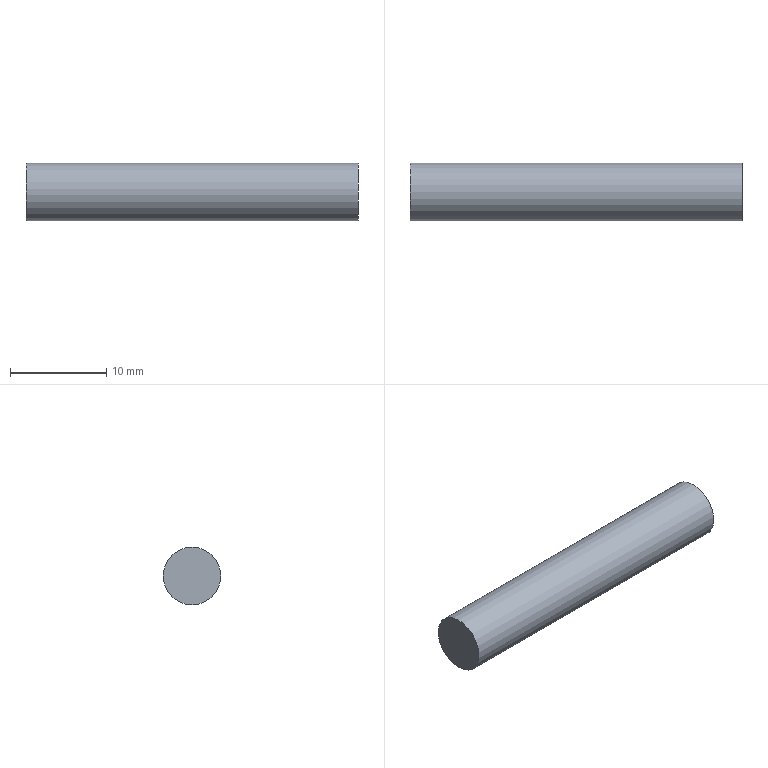Part | NX | features solid 2 | 1 solid | 3 faces | box 34.5 x 6 x 6 mm | volume 975.465 mm3 | plane 2 | cylinder 1 | commonest cylinder face diameters 6 x1
STEP:
#1=CARTESIAN_POINT('',(-125.,-72.,-32.));
#2=VERTEX_POINT('',#1);
#3=CARTESIAN_POINT('',(-125.,-72.,-35.));
#4=DIRECTION('',(-1.,0.,0.));
#5=DIRECTION('',(0.,0.,1.));
#6=AXIS2_PLACEMENT_3D('',#3,#4,#5);
#7=CIRCLE('',#6,3.);
#8=EDGE_CURVE('',#2,#2,#7,.F.);
#9=ORIENTED_EDGE('',*,*,#8,.T.);
#10=EDGE_LOOP('',(#9));
#11=FACE_BOUND('',#10,.T.);
#12=CARTESIAN_POINT('',(-90.5,-72.,-32.));
#13=VERTEX_POINT('',#12);
#14=CARTESIAN_POINT('',(-90.5,-72.,-35.));
#15=DIRECTION('',(-1.,0.,0.));
#16=DIRECTION('',(0.,0.,1.));
#17=AXIS2_PLACEMENT_3D('',#14,#15,#16);
#18=CIRCLE('',#17,3.);
#19=EDGE_CURVE('',#13,#13,#18,.F.);
#20=ORIENTED_EDGE('',*,*,#19,.F.);
#21=EDGE_LOOP('',(#20));
#22=FACE_BOUND('',#21,.T.);
#23=CARTESIAN_POINT('',(-125.,-72.,-35.));
#24=DIRECTION('',(1.,0.,0.));
#25=DIRECTION('',(0.,0.,1.));
#26=AXIS2_PLACEMENT_3D('',#23,#24,#25);
#27=CYLINDRICAL_SURFACE('',#26,3.);
#28=ADVANCED_FACE('',(#11,#22),#27,.T.);
#29=ORIENTED_EDGE('',*,*,#8,.F.);
#30=EDGE_LOOP('',(#29));
#31=FACE_BOUND('',#30,.T.);
#32=CARTESIAN_POINT('',(-125.,-3.,-30.));
#33=DIRECTION('',(1.,0.,0.));
#34=DIRECTION('',(0.,0.,1.));
#35=AXIS2_PLACEMENT_3D('',#32,#33,#34);
#36=PLANE('',#35);
#37=ADVANCED_FACE('',(#31),#36,.F.);
#38=ORIENTED_EDGE('',*,*,#19,.T.);
#39=EDGE_LOOP('',(#38));
#40=FACE_BOUND('',#39,.T.);
#41=CARTESIAN_POINT('',(-90.5,-3.,-42.5));
#42=DIRECTION('',(1.,0.,0.));
#43=DIRECTION('',(0.,0.,1.));
#44=AXIS2_PLACEMENT_3D('',#41,#42,#43);
#45=PLANE('',#44);
#46=ADVANCED_FACE('',(#40),#45,.T.);
#47=CLOSED_SHELL('',(#28,#37,#46));
#48=MANIFOLD_SOLID_BREP('',#47);
#49=(LENGTH_UNIT()NAMED_UNIT(*)SI_UNIT(.MILLI.,.METRE.));
#50=UNCERTAINTY_MEASURE_WITH_UNIT(LENGTH_MEASURE(0.00001),#49,'','');
#51=(NAMED_UNIT(*)PLANE_ANGLE_UNIT()SI_UNIT($,.RADIAN.));
#52=(NAMED_UNIT(*)SI_UNIT($,.STERADIAN.)SOLID_ANGLE_UNIT());
#53=(GEOMETRIC_REPRESENTATION_CONTEXT(3)GLOBAL_UNCERTAINTY_ASSIGNED_CONTEXT((#50))GLOBAL_UNIT_ASSIGNED_CONTEXT((#49,#51,#52))REPRESENTATION_CONTEXT('',''));
#54=ADVANCED_BREP_SHAPE_REPRESENTATION('',(#48),#53);